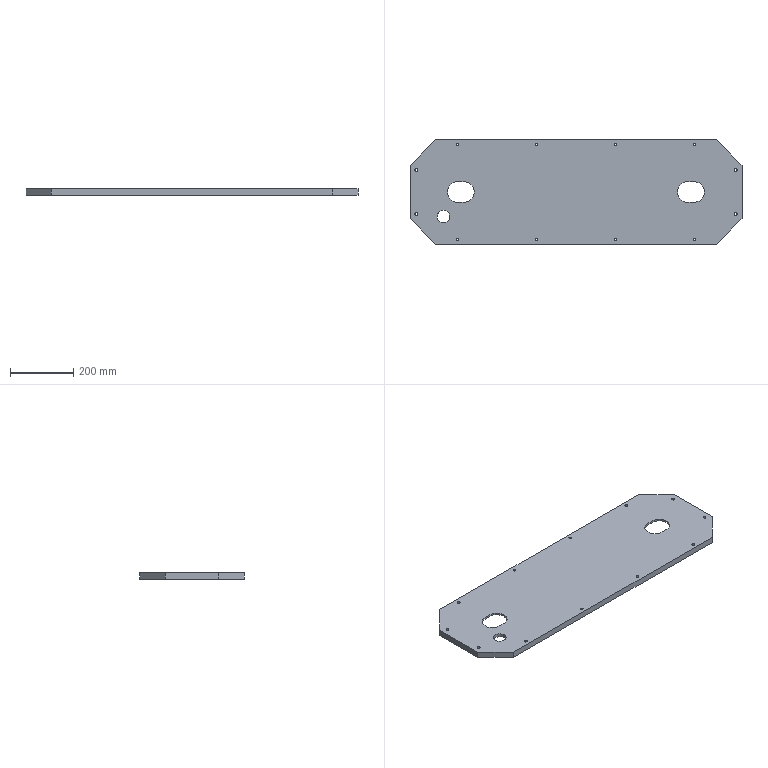Part | SolidWorks | features BaseBody 1 | 1 solid | 112 faces | box 1050 x 330 x 20 mm | volume 5286047 mm3 | cylinder 72 | plane 40 | commonest cylinder face diameters 9 x24 15 x24 65 x6 110 x6 10 x4 190 x4